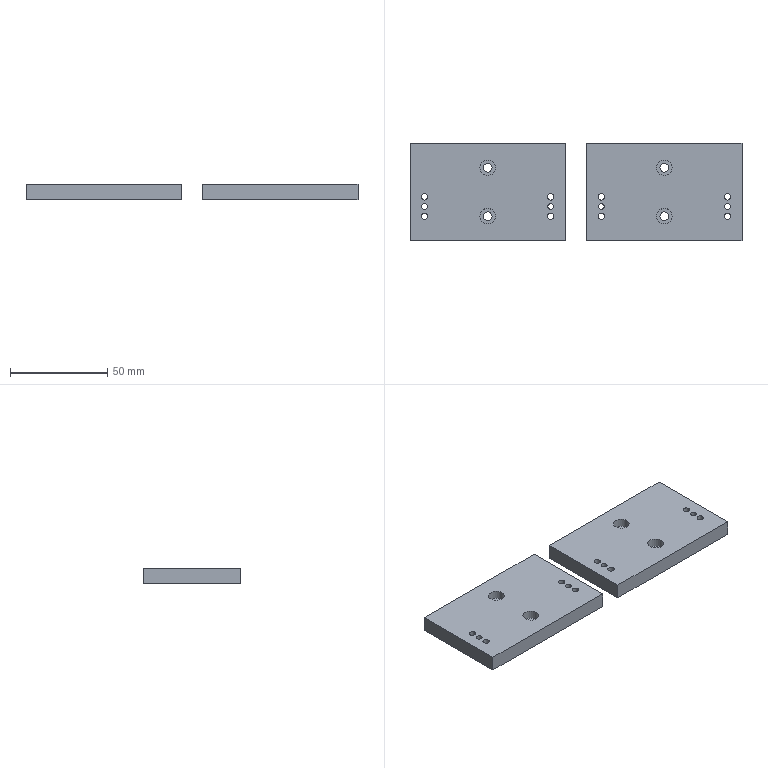CAM job | NX | 3-axis milling, drilling | part box 171 x 50 x 8 mm | stock box 176 x 55 x 10 mm
Tools:
number,name,description,diameter,corner_radius,flute_length,length,flutes
4,D4,平底铣刀-粗,4.0,0.0,25.0,75.0,2
9,D10,平底铣刀-粗,10.0,0.0,35.0,75.0,2
11,D4-J,平底铣刀-精,4.0,0.0,50.0,75.0,2
7,D6-J,平底铣刀-精,6.0,0.0,25.0,75.0,2
1,D80R0.8FLYCUTTER,圆鼻刀-粗,80.0,0.8,50.0,75.0,2
1,D80R0.8FLYCUTTER-J,圆鼻刀-精,80.0,0.8,50.0,75.0,2
2,D6CHAMFERMILL,倒角刀,6.0,0.0,3.0,25.0,2
21,M4X0.7,丝锥,3.3,0.0,35.0,50.0,2
18,D3REAMER,Drilling Tool,3.0,0.0,75.0,100.0,6
13,ZT3.4,钻头,3.4,0.0,35.0,50.0,2
11,ZT4.5,钻头,4.5,0.0,35.0,50.0,2
17,ZT2.9,Drilling Tool,2.9,0.0,35.0,50.0,2
Operations:
program,operation,operation_type,tool,method,geometry_group,spindle_rpm,surface_speed,feed_per_tooth,feed_cut,feed_plunge,cut_length_mm,path_length_mm,cut_time_min,machine_time_min
B,BOTTOMWALL_FACEROUGH1_COPY,VolumeBased25DMillingOperation,D80R0.8FLYCUTTER,ZLEVELROUGH-DEPTHK-STEPG,W-B,2800.0,703.696,0.5357,3000.0,100.0,1116.776,2036.734,0.3723,0.4643
B,BOTTOMWALL_FACEFINISH1_COPY,VolumeBased25DMillingOperation,D80R0.8FLYCUTTER-J,SIDEFINISH-DEPTHK-STEPG,W-B,4000.0,1005.28,0.125,1000.0,100.0,278.998,374.998,0.279,0.2886
B,COUNTERBOREMILL_1,CylinderMilling,D4,METHOD,W-B,8000.0,100.531,0.0375,600.0,100.0,152.006,446.406,0.2533,0.2828
B,COUNTERBOREMILL_2,CylinderMilling,D4,METHOD,W-B,8000.0,100.531,0.0375,600.0,100.0,152.006,446.406,0.2533,0.2828
B,NG_DRILLCHAMFER_3,Operation,D6CHAMFERMILL,METHOD,W-B,8000.0,150.796,0.0625,1000.0,0.0,19.2,303.711,0.0192,0.0477
B,NG_DRILLCHAMFER_4,Operation,D6CHAMFERMILL,METHOD,W-B,8000.0,150.796,0.0625,1000.0,0.0,41.6,402.272,0.0416,0.0777
B,CHAMFERMILL_2,PlanarMilling,D6CHAMFERMILL,METHOD,W-B,8000.0,150.796,0.0375,600.0,100.0,47.132,600.134,0.0786,0.1339
B,PLANEDEBURR6X45L_COPY,SurfaceContour,D6CHAMFERMILL,WALLCHAMFER-DEPTH0-STEPG,W-B,6500.0,122.519,0.1154,1500.0,100.0,700.411,1454.025,0.4669,0.5423
B,HOLEMILL_1,CylinderMilling,D4-J,METHOD,W-B,8000.0,100.531,0.0125,200.0,100.0,18.89,317.89,0.0945,0.1244
B,HOLEMILL_2,CylinderMilling,D4-J,METHOD,W-B,8000.0,100.531,0.0125,200.0,100.0,18.89,317.89,0.0945,0.1244
A,TOPFACE,FaceMilling,D80R0.8FLYCUTTER,SIDEFINISH-DEPTHK-STEPG,W-A,4500.0,1385.0,0.1667,1500.0,100.0,265.0,361.0,0.1767,0.1863
A,CONTOURROUGH_2,VolumeBased25DMillingOperation,D10,METHOD,W-A,8000.0,251.327,0.375,6000.0,80.0,7012.084,7316.584,1.169,1.199
A,SPOTDRILL-DEPTH0.8,Operation,D6CHAMFERMILL,NONE,W-A,8000.0,150.796,0.0312,500.0,90.0,28.8,426.099,0.0576,0.0973
A,THROUGH-PRECISION3.0PREDRILL,Operation,ZT2.9,NONE,W-A,3200.0,29.154,0.0312,200.0,90.0,51.349,361.732,0.2567,0.2878
A,THROUGH-M4TAPDRILL,Operation,ZT3.4,NONE,W-A,3000.0,31.102,0.05,300.0,90.0,120.0,543.234,0.4,0.4423
A,COUNTERBORE-DRILL0SEG,Operation,ZT4.5,NONE,W-A,2800.0,39.584,0.0179,100.0,90.0,48.0,340.046,0.48,0.5092
A,HOLEROUGHD4_1,CylinderMilling,D4,NONE,W-A,8000.0,100.531,0.075,1200.0,100.0,851.827,1408.427,0.7099,0.7655
A,HOLEFINISHD4_1,CylinderMilling,D4-J,FINISHSTEPDEPTHOFF,W-A,8000.0,100.531,0.0312,500.0,100.0,128.184,684.784,0.2564,0.312
A,SELECTSOLIDONLY,SurfaceContour,D6CHAMFERMILL,METHOD,W-A,8000.0,150.796,0.1875,3000.0,100.0,554.63,837.731,0.1849,0.2132
A,NG_DRILLCHAMFER_1,Operation,D6CHAMFERMILL,METHOD,W-A,8000.0,150.796,0.0312,500.0,0.0,19.2,303.711,0.0384,0.0669
A,NG_DRILLCHAMFER_2,Operation,D6CHAMFERMILL,METHOD,W-A,8000.0,150.796,0.0312,500.0,0.0,41.6,402.272,0.0832,0.1193
A,CHAMFERMILL_1,PlanarMilling,D6CHAMFERMILL,NONE,W-A,8000.0,150.796,0.0312,500.0,100.0,135.871,656.06,0.2717,0.3238
A,REAM,Operation,D3REAMER,METHOD,W-A,500.0,4.712,0.0167,50.0,0.0,40.0,339.035,0.8,0.8299
A,THROUGH-TAPM4,Operation,M4X0.7,METHOD,W-A,600.0,6.22,0.0006,0.7,90.0,96.0,495.234,137.143,137.183
A,CONTOURSEMI_2,VolumeBased25DMillingOperation,D6-J,METHOD,W-A,9000.0,169.646,0.0667,1200.0,100.0,567.532,891.049,0.4729,0.5053